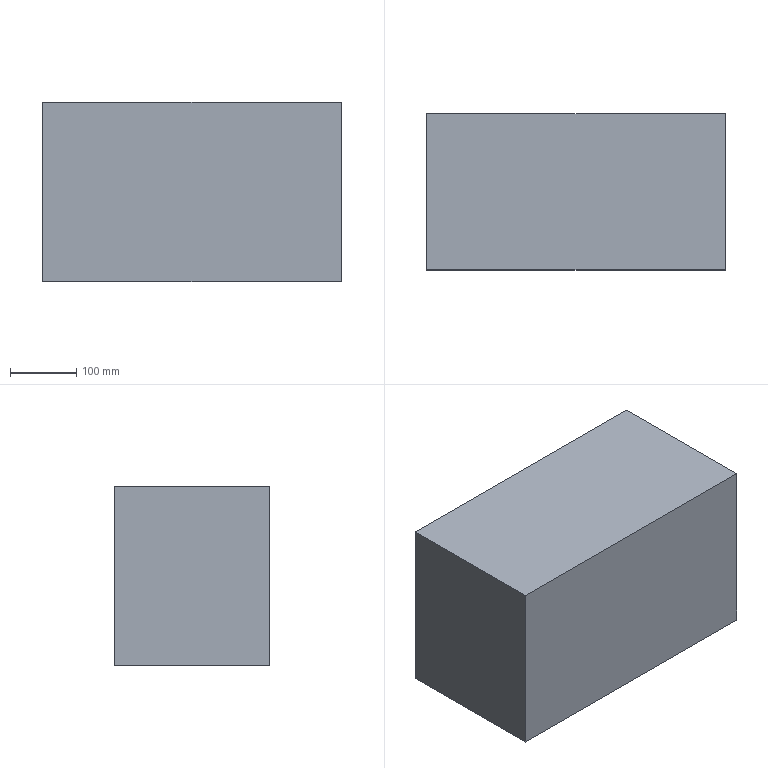Part | STEP file | zhichentai | 1 solid | 6 faces | box 450 x 234.83 x 270 mm | volume 28531845 mm3 | plane 6
STEP:
#1=CARTESIAN_POINT('',(0.,0.,0.));
#2=DIRECTION('',(0.,0.,1.));
#3=DIRECTION('',(1.,0.,0.));
#4=AXIS2_PLACEMENT_3D('',#1,#2,#3);
#5=CARTESIAN_POINT('',(0.,-117.415,0.));
#6=VERTEX_POINT('',#5);
#7=CARTESIAN_POINT('',(0.,-117.415,270.));
#8=VERTEX_POINT('',#7);
#9=CARTESIAN_POINT('',(0.,-117.415,270.));
#10=DIRECTION('',(0.,0.,1.));
#11=VECTOR('',#10,1.);
#12=LINE('',#9,#11);
#13=CARTESIAN_POINT('',(0.,117.415,270.));
#14=DIRECTION('',(1.,0.,0.));
#15=DIRECTION('',(0.,0.,-1.));
#16=AXIS2_PLACEMENT_3D('',#13,#14,#15);
#17=PLANE('',#16);
#18=CARTESIAN_POINT('',(0.,-234.83));
#19=DIRECTION('',(-1.,0.));
#20=VECTOR('',#19,1.);
#21=LINE('',#18,#20);
#22=(GEOMETRIC_REPRESENTATION_CONTEXT(2)PARAMETRIC_REPRESENTATION_CONTEXT()REPRESENTATION_CONTEXT('',''));
#23=DEFINITIONAL_REPRESENTATION('',(#21),#22);
#24=PCURVE('',#17,#23);
#25=CARTESIAN_POINT('',(0.,-117.415,0.));
#26=DIRECTION('',(0.,-1.,0.));
#27=DIRECTION('',(0.,0.,-1.));
#28=AXIS2_PLACEMENT_3D('',#25,#26,#27);
#29=PLANE('',#28);
#30=CARTESIAN_POINT('',(-270.,0.));
#31=DIRECTION('',(-1.,0.));
#32=VECTOR('',#31,1.);
#33=LINE('',#30,#32);
#34=(GEOMETRIC_REPRESENTATION_CONTEXT(2)PARAMETRIC_REPRESENTATION_CONTEXT()REPRESENTATION_CONTEXT('',''));
#35=DEFINITIONAL_REPRESENTATION('',(#33),#34);
#36=PCURVE('',#29,#35);
#37=SURFACE_CURVE('',#12,(#24,#36),.PCURVE_S1.);
#38=EDGE_CURVE('',#6,#8,#37,.T.);
#39=ORIENTED_EDGE('',*,*,#38,.T.);
#40=CARTESIAN_POINT('',(0.,117.415,270.));
#41=VERTEX_POINT('',#40);
#42=CARTESIAN_POINT('',(0.,117.415,270.));
#43=DIRECTION('',(0.,-1.,0.));
#44=VECTOR('',#43,1.);
#45=LINE('',#42,#44);
#46=CARTESIAN_POINT('',(0.,0.));
#47=DIRECTION('',(0.,-1.));
#48=VECTOR('',#47,1.);
#49=LINE('',#46,#48);
#50=(GEOMETRIC_REPRESENTATION_CONTEXT(2)PARAMETRIC_REPRESENTATION_CONTEXT()REPRESENTATION_CONTEXT('',''));
#51=DEFINITIONAL_REPRESENTATION('',(#49),#50);
#52=PCURVE('',#17,#51);
#53=CARTESIAN_POINT('',(450.,117.415,270.));
#54=DIRECTION('',(0.,0.,-1.));
#55=DIRECTION('',(-1.,0.,0.));
#56=AXIS2_PLACEMENT_3D('',#53,#54,#55);
#57=PLANE('',#56);
#58=CARTESIAN_POINT('',(450.,0.));
#59=DIRECTION('',(0.,-1.));
#60=VECTOR('',#59,1.);
#61=LINE('',#58,#60);
#62=(GEOMETRIC_REPRESENTATION_CONTEXT(2)PARAMETRIC_REPRESENTATION_CONTEXT()REPRESENTATION_CONTEXT('',''));
#63=DEFINITIONAL_REPRESENTATION('',(#61),#62);
#64=PCURVE('',#57,#63);
#65=SURFACE_CURVE('',#45,(#52,#64),.PCURVE_S1.);
#66=EDGE_CURVE('',#41,#8,#65,.T.);
#67=ORIENTED_EDGE('',*,*,#66,.F.);
#68=CARTESIAN_POINT('',(0.,117.415,0.));
#69=VERTEX_POINT('',#68);
#70=CARTESIAN_POINT('',(0.,117.415,270.));
#71=DIRECTION('',(0.,0.,1.));
#72=VECTOR('',#71,1.);
#73=LINE('',#70,#72);
#74=CARTESIAN_POINT('',(0.,0.));
#75=DIRECTION('',(-1.,0.));
#76=VECTOR('',#75,1.);
#77=LINE('',#74,#76);
#78=(GEOMETRIC_REPRESENTATION_CONTEXT(2)PARAMETRIC_REPRESENTATION_CONTEXT()REPRESENTATION_CONTEXT('',''));
#79=DEFINITIONAL_REPRESENTATION('',(#77),#78);
#80=PCURVE('',#17,#79);
#81=CARTESIAN_POINT('',(0.,117.415,0.));
#82=DIRECTION('',(0.,-1.,0.));
#83=DIRECTION('',(0.,0.,-1.));
#84=AXIS2_PLACEMENT_3D('',#81,#82,#83);
#85=PLANE('',#84);
#86=CARTESIAN_POINT('',(-270.,0.));
#87=DIRECTION('',(-1.,0.));
#88=VECTOR('',#87,1.);
#89=LINE('',#86,#88);
#90=(GEOMETRIC_REPRESENTATION_CONTEXT(2)PARAMETRIC_REPRESENTATION_CONTEXT()REPRESENTATION_CONTEXT('',''));
#91=DEFINITIONAL_REPRESENTATION('',(#89),#90);
#92=PCURVE('',#85,#91);
#93=SURFACE_CURVE('',#73,(#80,#92),.PCURVE_S1.);
#94=EDGE_CURVE('',#69,#41,#93,.T.);
#95=ORIENTED_EDGE('',*,*,#94,.F.);
#96=CARTESIAN_POINT('',(0.,117.415,0.));
#97=DIRECTION('',(0.,-1.,0.));
#98=VECTOR('',#97,1.);
#99=LINE('',#96,#98);
#100=CARTESIAN_POINT('',(270.,0.));
#101=DIRECTION('',(0.,-1.));
#102=VECTOR('',#101,1.);
#103=LINE('',#100,#102);
#104=(GEOMETRIC_REPRESENTATION_CONTEXT(2)PARAMETRIC_REPRESENTATION_CONTEXT()REPRESENTATION_CONTEXT('',''));
#105=DEFINITIONAL_REPRESENTATION('',(#103),#104);
#106=PCURVE('',#17,#105);
#107=CARTESIAN_POINT('',(0.,117.415,0.));
#108=DIRECTION('',(0.,0.,1.));
#109=DIRECTION('',(1.,0.,0.));
#110=AXIS2_PLACEMENT_3D('',#107,#108,#109);
#111=PLANE('',#110);
#112=CARTESIAN_POINT('',(0.,0.));
#113=DIRECTION('',(0.,-1.));
#114=VECTOR('',#113,1.);
#115=LINE('',#112,#114);
#116=(GEOMETRIC_REPRESENTATION_CONTEXT(2)PARAMETRIC_REPRESENTATION_CONTEXT()REPRESENTATION_CONTEXT('',''));
#117=DEFINITIONAL_REPRESENTATION('',(#115),#116);
#118=PCURVE('',#111,#117);
#119=SURFACE_CURVE('',#99,(#106,#118),.PCURVE_S1.);
#120=EDGE_CURVE('',#69,#6,#119,.T.);
#121=ORIENTED_EDGE('',*,*,#120,.T.);
#122=EDGE_LOOP('',(#39,#67,#95,#121));
#123=FACE_BOUND('',#122,.T.);
#124=ADVANCED_FACE('',(#123),#17,.F.);
#125=CARTESIAN_POINT('',(450.,-117.415,270.));
#126=VERTEX_POINT('',#125);
#127=CARTESIAN_POINT('',(450.,-117.415,270.));
#128=DIRECTION('',(1.,0.,0.));
#129=VECTOR('',#128,1.);
#130=LINE('',#127,#129);
#131=CARTESIAN_POINT('',(0.,-234.83));
#132=DIRECTION('',(-1.,0.));
#133=VECTOR('',#132,1.);
#134=LINE('',#131,#133);
#135=(GEOMETRIC_REPRESENTATION_CONTEXT(2)PARAMETRIC_REPRESENTATION_CONTEXT()REPRESENTATION_CONTEXT('',''));
#136=DEFINITIONAL_REPRESENTATION('',(#134),#135);
#137=PCURVE('',#57,#136);
#138=CARTESIAN_POINT('',(-270.,450.));
#139=DIRECTION('',(0.,1.));
#140=VECTOR('',#139,1.);
#141=LINE('',#138,#140);
#142=(GEOMETRIC_REPRESENTATION_CONTEXT(2)PARAMETRIC_REPRESENTATION_CONTEXT()REPRESENTATION_CONTEXT('',''));
#143=DEFINITIONAL_REPRESENTATION('',(#141),#142);
#144=PCURVE('',#29,#143);
#145=SURFACE_CURVE('',#130,(#137,#144),.PCURVE_S1.);
#146=EDGE_CURVE('',#8,#126,#145,.T.);
#147=ORIENTED_EDGE('',*,*,#146,.T.);
#148=CARTESIAN_POINT('',(450.,117.415,270.));
#149=VERTEX_POINT('',#148);
#150=CARTESIAN_POINT('',(450.,117.415,270.));
#151=DIRECTION('',(0.,-1.,0.));
#152=VECTOR('',#151,1.);
#153=LINE('',#150,#152);
#154=CARTESIAN_POINT('',(0.,0.));
#155=DIRECTION('',(0.,-1.));
#156=VECTOR('',#155,1.);
#157=LINE('',#154,#156);
#158=(GEOMETRIC_REPRESENTATION_CONTEXT(2)PARAMETRIC_REPRESENTATION_CONTEXT()REPRESENTATION_CONTEXT('',''));
#159=DEFINITIONAL_REPRESENTATION('',(#157),#158);
#160=PCURVE('',#57,#159);
#161=CARTESIAN_POINT('',(450.,117.415,0.));
#162=DIRECTION('',(-1.,0.,0.));
#163=DIRECTION('',(0.,0.,1.));
#164=AXIS2_PLACEMENT_3D('',#161,#162,#163);
#165=PLANE('',#164);
#166=CARTESIAN_POINT('',(270.,0.));
#167=DIRECTION('',(0.,-1.));
#168=VECTOR('',#167,1.);
#169=LINE('',#166,#168);
#170=(GEOMETRIC_REPRESENTATION_CONTEXT(2)PARAMETRIC_REPRESENTATION_CONTEXT()REPRESENTATION_CONTEXT('',''));
#171=DEFINITIONAL_REPRESENTATION('',(#169),#170);
#172=PCURVE('',#165,#171);
#173=SURFACE_CURVE('',#153,(#160,#172),.PCURVE_S1.);
#174=EDGE_CURVE('',#149,#126,#173,.T.);
#175=ORIENTED_EDGE('',*,*,#174,.F.);
#176=CARTESIAN_POINT('',(450.,117.415,270.));
#177=DIRECTION('',(1.,0.,0.));
#178=VECTOR('',#177,1.);
#179=LINE('',#176,#178);
#180=CARTESIAN_POINT('',(0.,0.));
#181=DIRECTION('',(-1.,0.));
#182=VECTOR('',#181,1.);
#183=LINE('',#180,#182);
#184=(GEOMETRIC_REPRESENTATION_CONTEXT(2)PARAMETRIC_REPRESENTATION_CONTEXT()REPRESENTATION_CONTEXT('',''));
#185=DEFINITIONAL_REPRESENTATION('',(#183),#184);
#186=PCURVE('',#57,#185);
#187=CARTESIAN_POINT('',(-270.,450.));
#188=DIRECTION('',(0.,1.));
#189=VECTOR('',#188,1.);
#190=LINE('',#187,#189);
#191=(GEOMETRIC_REPRESENTATION_CONTEXT(2)PARAMETRIC_REPRESENTATION_CONTEXT()REPRESENTATION_CONTEXT('',''));
#192=DEFINITIONAL_REPRESENTATION('',(#190),#191);
#193=PCURVE('',#85,#192);
#194=SURFACE_CURVE('',#179,(#186,#193),.PCURVE_S1.);
#195=EDGE_CURVE('',#41,#149,#194,.T.);
#196=ORIENTED_EDGE('',*,*,#195,.F.);
#197=ORIENTED_EDGE('',*,*,#66,.T.);
#198=EDGE_LOOP('',(#147,#175,#196,#197));
#199=FACE_BOUND('',#198,.T.);
#200=ADVANCED_FACE('',(#199),#57,.F.);
#201=CARTESIAN_POINT('',(450.,-117.415,0.));
#202=VERTEX_POINT('',#201);
#203=CARTESIAN_POINT('',(450.,-117.415,0.));
#204=DIRECTION('',(0.,0.,-1.));
#205=VECTOR('',#204,1.);
#206=LINE('',#203,#205);
#207=CARTESIAN_POINT('',(0.,-234.83));
#208=DIRECTION('',(-1.,0.));
#209=VECTOR('',#208,1.);
#210=LINE('',#207,#209);
#211=(GEOMETRIC_REPRESENTATION_CONTEXT(2)PARAMETRIC_REPRESENTATION_CONTEXT()REPRESENTATION_CONTEXT('',''));
#212=DEFINITIONAL_REPRESENTATION('',(#210),#211);
#213=PCURVE('',#165,#212);
#214=CARTESIAN_POINT('',(0.,450.));
#215=DIRECTION('',(1.,0.));
#216=VECTOR('',#215,1.);
#217=LINE('',#214,#216);
#218=(GEOMETRIC_REPRESENTATION_CONTEXT(2)PARAMETRIC_REPRESENTATION_CONTEXT()REPRESENTATION_CONTEXT('',''));
#219=DEFINITIONAL_REPRESENTATION('',(#217),#218);
#220=PCURVE('',#29,#219);
#221=SURFACE_CURVE('',#206,(#213,#220),.PCURVE_S1.);
#222=EDGE_CURVE('',#126,#202,#221,.T.);
#223=ORIENTED_EDGE('',*,*,#222,.T.);
#224=CARTESIAN_POINT('',(450.,117.415,0.));
#225=VERTEX_POINT('',#224);
#226=CARTESIAN_POINT('',(450.,117.415,0.));
#227=DIRECTION('',(0.,-1.,0.));
#228=VECTOR('',#227,1.);
#229=LINE('',#226,#228);
#230=CARTESIAN_POINT('',(0.,0.));
#231=DIRECTION('',(0.,-1.));
#232=VECTOR('',#231,1.);
#233=LINE('',#230,#232);
#234=(GEOMETRIC_REPRESENTATION_CONTEXT(2)PARAMETRIC_REPRESENTATION_CONTEXT()REPRESENTATION_CONTEXT('',''));
#235=DEFINITIONAL_REPRESENTATION('',(#233),#234);
#236=PCURVE('',#165,#235);
#237=CARTESIAN_POINT('',(450.,0.));
#238=DIRECTION('',(0.,-1.));
#239=VECTOR('',#238,1.);
#240=LINE('',#237,#239);
#241=(GEOMETRIC_REPRESENTATION_CONTEXT(2)PARAMETRIC_REPRESENTATION_CONTEXT()REPRESENTATION_CONTEXT('',''));
#242=DEFINITIONAL_REPRESENTATION('',(#240),#241);
#243=PCURVE('',#111,#242);
#244=SURFACE_CURVE('',#229,(#236,#243),.PCURVE_S1.);
#245=EDGE_CURVE('',#225,#202,#244,.T.);
#246=ORIENTED_EDGE('',*,*,#245,.F.);
#247=CARTESIAN_POINT('',(450.,117.415,0.));
#248=DIRECTION('',(0.,0.,-1.));
#249=VECTOR('',#248,1.);
#250=LINE('',#247,#249);
#251=CARTESIAN_POINT('',(0.,0.));
#252=DIRECTION('',(-1.,0.));
#253=VECTOR('',#252,1.);
#254=LINE('',#251,#253);
#255=(GEOMETRIC_REPRESENTATION_CONTEXT(2)PARAMETRIC_REPRESENTATION_CONTEXT()REPRESENTATION_CONTEXT('',''));
#256=DEFINITIONAL_REPRESENTATION('',(#254),#255);
#257=PCURVE('',#165,#256);
#258=CARTESIAN_POINT('',(0.,450.));
#259=DIRECTION('',(1.,0.));
#260=VECTOR('',#259,1.);
#261=LINE('',#258,#260);
#262=(GEOMETRIC_REPRESENTATION_CONTEXT(2)PARAMETRIC_REPRESENTATION_CONTEXT()REPRESENTATION_CONTEXT('',''));
#263=DEFINITIONAL_REPRESENTATION('',(#261),#262);
#264=PCURVE('',#85,#263);
#265=SURFACE_CURVE('',#250,(#257,#264),.PCURVE_S1.);
#266=EDGE_CURVE('',#149,#225,#265,.T.);
#267=ORIENTED_EDGE('',*,*,#266,.F.);
#268=ORIENTED_EDGE('',*,*,#174,.T.);
#269=EDGE_LOOP('',(#223,#246,#267,#268));
#270=FACE_BOUND('',#269,.T.);
#271=ADVANCED_FACE('',(#270),#165,.F.);
#272=CARTESIAN_POINT('',(0.,-117.415,0.));
#273=DIRECTION('',(-1.,0.,0.));
#274=VECTOR('',#273,1.);
#275=LINE('',#272,#274);
#276=CARTESIAN_POINT('',(0.,-234.83));
#277=DIRECTION('',(-1.,0.));
#278=VECTOR('',#277,1.);
#279=LINE('',#276,#278);
#280=(GEOMETRIC_REPRESENTATION_CONTEXT(2)PARAMETRIC_REPRESENTATION_CONTEXT()REPRESENTATION_CONTEXT('',''));
#281=DEFINITIONAL_REPRESENTATION('',(#279),#280);
#282=PCURVE('',#111,#281);
#283=CARTESIAN_POINT('',(0.,0.));
#284=DIRECTION('',(0.,-1.));
#285=VECTOR('',#284,1.);
#286=LINE('',#283,#285);
#287=(GEOMETRIC_REPRESENTATION_CONTEXT(2)PARAMETRIC_REPRESENTATION_CONTEXT()REPRESENTATION_CONTEXT('',''));
#288=DEFINITIONAL_REPRESENTATION('',(#286),#287);
#289=PCURVE('',#29,#288);
#290=SURFACE_CURVE('',#275,(#282,#289),.PCURVE_S1.);
#291=EDGE_CURVE('',#202,#6,#290,.T.);
#292=ORIENTED_EDGE('',*,*,#291,.T.);
#293=ORIENTED_EDGE('',*,*,#120,.F.);
#294=CARTESIAN_POINT('',(0.,117.415,0.));
#295=DIRECTION('',(-1.,0.,0.));
#296=VECTOR('',#295,1.);
#297=LINE('',#294,#296);
#298=CARTESIAN_POINT('',(0.,0.));
#299=DIRECTION('',(-1.,0.));
#300=VECTOR('',#299,1.);
#301=LINE('',#298,#300);
#302=(GEOMETRIC_REPRESENTATION_CONTEXT(2)PARAMETRIC_REPRESENTATION_CONTEXT()REPRESENTATION_CONTEXT('',''));
#303=DEFINITIONAL_REPRESENTATION('',(#301),#302);
#304=PCURVE('',#111,#303);
#305=CARTESIAN_POINT('',(0.,0.));
#306=DIRECTION('',(0.,-1.));
#307=VECTOR('',#306,1.);
#308=LINE('',#305,#307);
#309=(GEOMETRIC_REPRESENTATION_CONTEXT(2)PARAMETRIC_REPRESENTATION_CONTEXT()REPRESENTATION_CONTEXT('',''));
#310=DEFINITIONAL_REPRESENTATION('',(#308),#309);
#311=PCURVE('',#85,#310);
#312=SURFACE_CURVE('',#297,(#304,#311),.PCURVE_S1.);
#313=EDGE_CURVE('',#225,#69,#312,.T.);
#314=ORIENTED_EDGE('',*,*,#313,.F.);
#315=ORIENTED_EDGE('',*,*,#245,.T.);
#316=EDGE_LOOP('',(#292,#293,#314,#315));
#317=FACE_BOUND('',#316,.T.);
#318=ADVANCED_FACE('',(#317),#111,.F.);
#319=ORIENTED_EDGE('',*,*,#94,.T.);
#320=ORIENTED_EDGE('',*,*,#195,.T.);
#321=ORIENTED_EDGE('',*,*,#266,.T.);
#322=ORIENTED_EDGE('',*,*,#313,.T.);
#323=EDGE_LOOP('',(#319,#320,#321,#322));
#324=FACE_BOUND('',#323,.T.);
#325=ADVANCED_FACE('',(#324),#85,.F.);
#326=ORIENTED_EDGE('',*,*,#38,.F.);
#327=ORIENTED_EDGE('',*,*,#291,.F.);
#328=ORIENTED_EDGE('',*,*,#222,.F.);
#329=ORIENTED_EDGE('',*,*,#146,.F.);
#330=EDGE_LOOP('',(#326,#327,#328,#329));
#331=FACE_BOUND('',#330,.T.);
#332=ADVANCED_FACE('',(#331),#29,.T.);
#333=CLOSED_SHELL('',(#124,#200,#271,#318,#325,#332));
#334=MANIFOLD_SOLID_BREP('',#333);
#335=(LENGTH_UNIT()NAMED_UNIT(*)SI_UNIT(.MILLI.,.METRE.));
#336=UNCERTAINTY_MEASURE_WITH_UNIT(LENGTH_MEASURE(0.0000001),#335,'','');
#337=(NAMED_UNIT(*)PLANE_ANGLE_UNIT()SI_UNIT($,.RADIAN.));
#338=(NAMED_UNIT(*)SI_UNIT($,.STERADIAN.)SOLID_ANGLE_UNIT());
#339=(GEOMETRIC_REPRESENTATION_CONTEXT(3)GLOBAL_UNCERTAINTY_ASSIGNED_CONTEXT((#336))GLOBAL_UNIT_ASSIGNED_CONTEXT((#335,#337,#338))REPRESENTATION_CONTEXT('',''));
#340=ADVANCED_BREP_SHAPE_REPRESENTATION('',(#4,#334),#339);